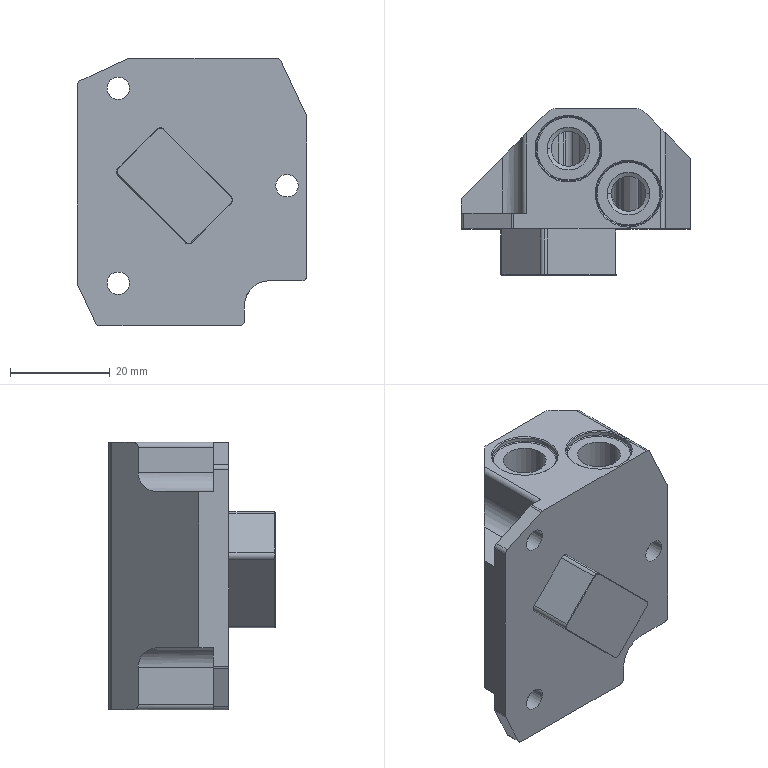NC program | NX | posted with a generic post | part box 46 x 33.25 x 53.5 mm
Whole program:
N10 G17 G21 G94 G90
(FLOOR_FACING , TOOL : D10-30-D10-75-3T-ROUGH)
N12 T02 M6
N14 G54
N16 G17 G0 G90 X17.268 Y3.406 B0. C0. S3500 M3
N18 G43 Z23. H2
N20 Z3.1 B-180. C-180.
N22 G94 G1 Z0.1 F1000.
N24 X15.859 Y4.766
N26 G3 X12.324 Y4.705 R2.5
N28 G1 X-9.076 Y-17.453
N30 X-13.763 Y-12.766
N32 X7.636 Y9.392
N34 G2 X11.171 Y9.454 R2.5
N36 G1 X11.494 Y9.777
N38 Z3.1
N40 G0 Z23.
(PLANAR_MILL_5_COPY , TOOL : D10-30-D10-75-3T-ROUGH)
N42 X-36.75 Y9.743
N44 Z10.85
N46 Z-6.15
N48 G1 Z-9.15
N50 X-26.75
N52 Y16.907
N54 G2 X-26.173 Y17.813 R1.
N56 G1 X-15.251 Y22.906
N58 G2 X-14.828 Y23. R1.
N60 G1 X16.75
N62 G2 X17.75 Y22. R1.
N64 G1 Y15.5
N66 G3 X22.75 Y10.5 R5.
N68 G1 X25.75
N70 G2 X26.75 Y9.5 R1.
N72 G1 Y-18.421
N74 G2 X26.173 Y-19.327 R1.
N76 G1 X18.497 Y-22.906
N78 G2 X18.074 Y-23. R1.
N80 G1 X-21.313
N82 G2 X-22.219 Y-22.423 R1.
N84 G1 X-26.656 Y-12.907
N86 G2 X-26.75 Y-12.485 R1.
N88 G1 Y9.743
N90 X-20.75
N92 Y13.722
N94 X-13.72 Y17.
N96 X11.75
N98 Y15.5
N100 G3 X20.75 Y4.683 R11.
N102 G1 Y-12.
N104 X15.641 Y-11.891
N106 X20.75 Y-12.
N108 Y-15.235
N110 X16.966 Y-17.
N112 X3.352
N114 X14.518 Y-5.833
N116 G3 X14.518 Y4.49 R7.3
N118 G1 X6.74 Y12.268
N120 G3 X-3.583 Y12.268 R7.3
N122 G1 X-17.018 Y-1.167
N124 G3 X-17.018 Y-11.49 R7.3
N126 G1 X-11.509 Y-17.
N128 X-10.66 Y-16.151
N130 X-16.17 Y-10.642
N132 G2 X-16.17 Y-2.015 R6.1
N134 G1 X-2.735 Y11.42
N136 G2 X5.892 Y11.42 R6.1
N138 G1 X13.67 Y3.642
N140 G2 X13.67 Y-4.985 R6.1
N142 G1 X0.235 Y-18.42
N144 G2 X-8.392 Y-18.42 R6.1
N146 G1 X-10.66 Y-16.151
N148 X-11.509 Y-17.
N150 X-18.128
N152 X-20.75 Y-11.376
N154 Y9.743
N156 X-14.75
N158 Y9.899
N160 X-14.165 Y10.172
N162 X-14.75 Y9.587
N164 Y9.743
N166 X-36.75
N168 Z-6.15
N170 G0 Z10.85
N172 M5
(HOLE_MILLING , TOOL : D3-9-D4-50-3T-ROUGH)
N174 T07 M6
N176 G54
N178 G17 G0 G90 X-1.25 Y19. B0. C0. S3000 M3
N180 G43 Z10.75 H7
N182 Z-8.25 B-180. C-180.
N184 G94 G3 X-0.875 Y19.375 R0.375 F400.
N186 X-1.25 Y19.75 R0.375
N188 X-1.25 Y19.75 Z-8.55 I0. J-0.75
N190 X-1.25 Y19.75 Z-8.85 I0. J-0.75
N192 X-1.25 Y19.75 Z-9.15 I0. J-0.75
N194 X-1.25 Y19.75 Z-9.45 I0. J-0.75
N196 X-1.25 Y19.75 Z-9.75 I0. J-0.75
N198 X-1.25 Y19.75 Z-10.05 I0. J-0.75
N200 X-1.25 Y19.75 Z-10.35 I0. J-0.75
N202 X-1.25 Y19.75 Z-10.65 I0. J-0.75
N204 X-1.25 Y19.75 Z-10.95 I0. J-0.75
N206 X-1.25 Y19.75 Z-11.25 I0. J-0.75
N208 X-1.25 Y19.75 Z-11.55 I0. J-0.75
N210 X-1.25 Y19.75 Z-11.85 I0. J-0.75
N212 X-1.25 Y19.75 Z-12.15 I0. J-0.75
N214 X-1.25 Y19.75 Z-12.45 I0. J-0.75
N216 X-1.25 Y19.75 Z-12.75 I0. J-0.75
N218 X-1.25 Y19.75 Z-13.05 I0. J-0.75
N220 X-0.6 Y18.625 Z-13.25 R-0.75
N222 X-0.875 Y19.65 R0.75
N224 X-0.6 Y18.625 R-0.75
N226 X-0.738 Y19.137 R0.375
N228 X-1.25 Y19. R0.375
N230 G0 Z10.75
N232 X18.236 Y-14.75
N234 Z-8.25
N236 G3 X18.611 Y-14.375 R0.375
N238 X18.236 Y-14. R0.375
N240 X18.236 Y-14. Z-8.55 I0. J-0.75
N242 X18.236 Y-14. Z-8.85 I0. J-0.75
N244 X18.236 Y-14. Z-9.15 I0. J-0.75
N246 X18.236 Y-14. Z-9.45 I0. J-0.75
N248 X18.236 Y-14. Z-9.75 I0. J-0.75
N250 X18.236 Y-14. Z-10.05 I0. J-0.75
N252 X18.236 Y-14. Z-10.35 I0. J-0.75
N254 X18.236 Y-14. Z-10.65 I0. J-0.75
N256 X18.236 Y-14. Z-10.95 I0. J-0.75
N258 X18.236 Y-14. Z-11.25 I0. J-0.75
N260 X18.236 Y-14. Z-11.55 I0. J-0.75
N262 X18.236 Y-14. Z-11.85 I0. J-0.75
N264 X18.236 Y-14. Z-12.15 I0. J-0.75
N266 X18.236 Y-14. Z-12.45 I0. J-0.75
N268 X18.236 Y-14. Z-12.75 I0. J-0.75
N270 X18.236 Y-14. Z-13.05 I0. J-0.75
N272 X18.885 Y-15.125 Z-13.25 R-0.75
N274 X18.611 Y-14.1 R0.75
N276 X18.885 Y-15.125 R-0.75
N278 X18.748 Y-14.613 R0.375
N280 X18.236 Y-14.75 R0.375
N282 G0 Z10.75
N284 X-20.736
N286 Z-8.25
N288 G3 X-20.361 Y-14.375 R0.375
N290 X-20.736 Y-14. R0.375
N292 X-20.736 Y-14. Z-8.55 I0. J-0.75
N294 X-20.736 Y-14. Z-8.85 I0. J-0.75
N296 X-20.736 Y-14. Z-9.15 I0. J-0.75
N298 X-20.736 Y-14. Z-9.45 I0. J-0.75
N300 X-20.736 Y-14. Z-9.75 I0. J-0.75
N302 X-20.736 Y-14. Z-10.05 I0. J-0.75
N304 X-20.736 Y-14. Z-10.35 I0. J-0.75
N306 X-20.736 Y-14. Z-10.65 I0. J-0.75
N308 X-20.736 Y-14. Z-10.95 I0. J-0.75
N310 X-20.736 Y-14. Z-11.25 I0. J-0.75
N312 X-20.736 Y-14. Z-11.55 I0. J-0.75
N314 X-20.736 Y-14. Z-11.85 I0. J-0.75
N316 X-20.736 Y-14. Z-12.15 I0. J-0.75
N318 X-20.736 Y-14. Z-12.45 I0. J-0.75
N320 X-20.736 Y-14. Z-12.75 I0. J-0.75
N322 X-20.736 Y-14. Z-13.05 I0. J-0.75
N324 X-20.086 Y-15.125 Z-13.25 R-0.75
N326 X-20.361 Y-14.1 R0.75
N328 X-20.086 Y-15.125 R-0.75
N330 X-20.223 Y-14.613 R0.375
N332 X-20.736 Y-14.75 R0.375
N334 G0 Z10.75
N336 M5
(FLOOR_FACING_1 , TOOL : D10-30-D10-75-3T-FINISH)
N338 T05 M6
N340 G54
N342 G17 G0 G90 X14.409 Y6.863 B0. C0. S3500 M3
N344 G43 Z23. H5
N346 Z3. B-180. C-180.
N348 G94 G1 Z0. F600.
N350 X12.324 Y4.705
N352 X-9.076 Y-17.453
N354 X-13.763 Y-12.766
N356 X7.636 Y9.392
N358 X9.721 Y11.551
N360 Z3.
N362 G0 Z23.
(PLANAR_MILL_5 , TOOL : D10-30-D10-75-3T-FINISH)
N364 X-36.75 Y9.673
N366 Z10.75
N368 Z-6.25
N370 G1 Z-9.25
N372 X-26.75
N374 Y16.907
N376 G2 X-26.173 Y17.813 R1.
N378 G1 X-15.251 Y22.906
N380 G2 X-14.828 Y23. R1.
N382 G1 X16.75
N384 G2 X17.75 Y22. R1.
N386 G1 Y15.5
N388 G3 X22.75 Y10.5 R5.
N390 G1 X25.75
N392 G2 X26.75 Y9.5 R1.
N394 G1 Y-18.421
N396 G2 X26.173 Y-19.327 R1.
N398 G1 X18.497 Y-22.906
N400 G2 X18.074 Y-23. R1.
N402 G1 X-21.313
N404 G2 X-22.219 Y-22.423 R1.
N406 G1 X-26.656 Y-12.907
N408 G2 X-26.75 Y-12.485 R1.
N410 G1 Y9.673
N412 X-20.75
N414 Y13.722
N416 X-13.72 Y17.
N418 X11.75
N420 Y15.5
N422 G3 X20.75 Y4.683 R11.
N424 G1 Y-12.
N426 X15.594 Y-11.844
N428 X20.75 Y-12.
N430 Y-15.235
N432 X16.966 Y-17.
N434 X3.211
N436 X14.448 Y-5.763
N438 G3 X14.448 Y4.42 R7.2
N440 G1 X6.67 Y12.198
N442 G3 X-3.513 Y12.198 R7.2
N444 G1 X-16.948 Y-1.237
N446 G3 X-16.948 Y-11.42 R7.2
N448 G1 X-11.367 Y-17.
N450 X-10.519 Y-16.151
N452 X-16.099 Y-10.571
N454 G2 X-16.099 Y-2.086 R6.
N456 G1 X-2.664 Y11.349
N458 G2 X5.821 Y11.349 R6.
N460 G1 X13.599 Y3.571
N462 G2 X13.599 Y-4.914 R6.
N464 G1 X0.164 Y-18.349
N466 G2 X-8.321 Y-18.349 R6.
N468 G1 X-10.519 Y-16.151
N470 X-11.367 Y-17.
N472 X-18.128
N474 X-20.75 Y-11.376
N476 Y9.673
N478 X-14.75
N480 Y9.899
N482 X-13.9 Y10.296
N484 X-14.75 Y9.446
N486 Y9.673
N488 X-36.75
N490 Z-6.25
N492 G0 Z10.75
(PLANAR_MILL_3 , TOOL : D10-30-D10-75-3T-FINISH)
N494 Z20.
N496 X-8.321 Y-21.178
N498 Z-7.245
N500 G1 Z-9.245
N502 G3 X-8.321 Y-18.349 R2.
N504 G1 X-16.099 Y-10.571
N506 G2 X-16.099 Y-2.086 R6.
N508 G1 X-2.664 Y11.349
N510 G2 X5.821 Y11.349 R6.
N512 G1 X13.599 Y3.571
N514 G2 X13.599 Y-4.914 R6.
N516 G1 X0.164 Y-18.349
N518 G2 X-8.321 Y-18.349 R6.
N520 G3 X-11.149 Y-18.349 R2.
N522 G1 Z-7.245
N524 G0 Z20.
N526 M5
(PLANAR_MILL_3_COPY , TOOL : 倒角D4-90度)
N528 T08 M6
N530 G54
N532 G17 G0 G90 X7.232 Y-9.153 B0. C0. S3500 M3
N534 G43 Z20. H8
N536 Z0.505 B-180. C-180.
N538 G94 G1 Z-1.495 F1000.
N540 G3 X4.403 Y-9.153 R2.
N542 G1 X-2.314 Y-15.871
N544 G2 X-5.843 Y-15.871 R2.495
N546 G1 X-13.621 Y-8.093
N548 G2 X-13.621 Y-4.564 R2.495
N550 G1 X-0.186 Y8.871
N552 G2 X3.343 Y8.871 R2.495
N554 G1 X11.121 Y1.093
N556 G2 X11.121 Y-2.436 R2.495
N558 G1 X4.403 Y-9.153
N560 G3 X4.403 Y-11.982 R2.
N562 G1 Z0.505
N564 G0 Z20.
(PLANAR_MILL_3_COPY_COPY , TOOL : 倒角D4-90度)
N566 X0.381 Y-26.495
N568 Z10.75
N570 Z-8.745
N572 G1 Z-10.745
N574 G3 X-1.619 Y-24.495 R2.
N576 G1 X-21.313
N578 G2 X-23.574 Y-23.054 R2.495
N580 G1 X-28.011 Y-13.539
N582 G2 X-28.245 Y-12.485 R2.495
N584 G1 Y16.907
N586 G2 X-26.804 Y19.168 R2.495
N588 G1 X-15.883 Y24.261
N590 G2 X-14.828 Y24.495 R2.495
N592 G1 X16.75
N594 G2 X19.245 Y22. R2.495
N596 G1 Y15.5
N598 G3 X22.75 Y11.995 R3.505
N600 G1 X25.75
N602 G2 X28.245 Y9.5 R2.495
N604 G1 Y-18.421
N606 G2 X26.804 Y-20.682 R2.495
N608 G1 X19.129 Y-24.261
N610 G2 X18.074 Y-24.495 R2.495
N612 G1 X-1.619
N614 G3 X-3.619 Y-26.495 R2.
N616 G1 Z-8.745
N618 G0 Z10.75
(PLANAR_MILL_3_COPY_COPY_1 , TOOL : 倒角D4-90度)
N620 X18.036 Y-15.268
N622 Z-8.745
N624 G1 Z-10.745
N626 Y-15.305
N628 G3 X18.236 Y-15.505 R0.2
N630 X18.991 Y-14.75 R0.755
N632 X18.236 Y-15.505 R-0.755
N634 X18.436 Y-15.305 R0.2
N636 G1 Y-15.268
N638 Z-8.745
N640 G0 Z10.75
N642 X-1.45 Y18.482
N644 Z-8.745
N646 G1 Z-10.745
N648 Y18.445
N650 G3 X-1.25 Y18.245 R0.2
N652 X-0.495 Y19. R0.755
N654 X-1.25 Y18.245 R-0.755
N656 X-1.05 Y18.445 R0.2
N658 G1 Y18.482
N660 Z-8.745
N662 G0 Z10.75
N664 X-20.936 Y-15.268
N666 Z-8.745
N668 G1 Z-10.745
N670 Y-15.305
N672 G3 X-20.736 Y-15.505 R0.2
N674 X-19.981 Y-14.75 R0.755
N676 X-20.736 Y-15.505 R-0.755
N678 X-20.536 Y-15.305 R0.2
N680 G1 Y-15.268
N682 Z-8.745
N684 G0 Z10.75
N686 M5
N688 M2